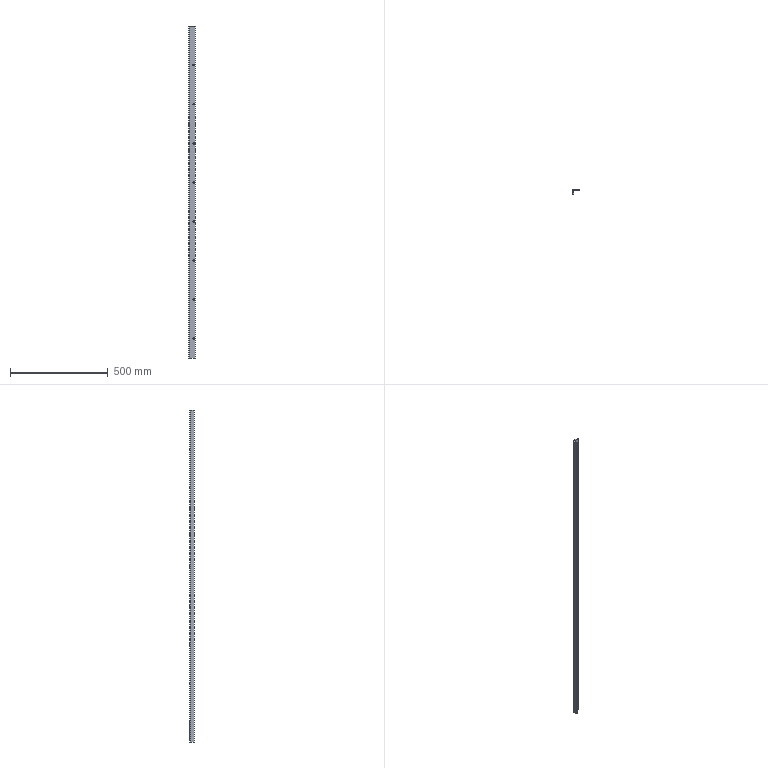Part | STEP file | Edge guard | 1 solid | 28 faces | box 35 x 25 x 1700 mm | volume 453852 mm3 | cylinder 19 | plane 9 | commonest cylinder face diameters 9 x17 1 x1 11 x1
STEP:
#1=CARTESIAN_POINT('',(7.,0.,-1895.5));
#2=VERTEX_POINT('',#1);
#3=CARTESIAN_POINT('',(7.,0.,-1904.5));
#4=VERTEX_POINT('',#3);
#5=CARTESIAN_POINT('',(7.,0.,-1900.));
#6=DIRECTION('',(0.,-1.,0.));
#7=DIRECTION('',(0.,0.,1.));
#8=AXIS2_PLACEMENT_3D('',#5,#6,#7);
#9=CIRCLE('',#8,4.5);
#10=EDGE_CURVE('',#2,#4,#9,.T.);
#11=ORIENTED_EDGE('',*,*,#10,.T.);
#12=CARTESIAN_POINT('',(7.,5.,-1904.5));
#13=VERTEX_POINT('',#12);
#14=CARTESIAN_POINT('',(7.,5.,-1904.5));
#15=DIRECTION('',(0.,1.,0.));
#16=VECTOR('',#15,1000.);
#17=LINE('',#14,#16);
#18=EDGE_CURVE('',#4,#13,#17,.T.);
#19=ORIENTED_EDGE('',*,*,#18,.T.);
#20=CARTESIAN_POINT('',(7.,5.,-1895.5));
#21=VERTEX_POINT('',#20);
#22=CARTESIAN_POINT('',(7.,5.,-1900.));
#23=DIRECTION('',(0.,-1.,0.));
#24=DIRECTION('',(0.,0.,1.));
#25=AXIS2_PLACEMENT_3D('',#22,#23,#24);
#26=CIRCLE('',#25,4.5);
#27=EDGE_CURVE('',#21,#13,#26,.T.);
#28=ORIENTED_EDGE('',*,*,#27,.F.);
#29=CARTESIAN_POINT('',(7.,5.,-1895.5));
#30=DIRECTION('',(0.,1.,0.));
#31=VECTOR('',#30,1000.);
#32=LINE('',#29,#31);
#33=EDGE_CURVE('',#2,#21,#32,.T.);
#34=ORIENTED_EDGE('',*,*,#33,.F.);
#35=EDGE_LOOP('',(#11,#19,#28,#34));
#36=FACE_OUTER_BOUND('',#35,.T.);
#37=CARTESIAN_POINT('',(7.,5.,-1900.));
#38=DIRECTION('',(0.,1.,0.));
#39=DIRECTION('',(0.,0.,1.));
#40=AXIS2_PLACEMENT_3D('',#37,#38,#39);
#41=CYLINDRICAL_SURFACE('',#40,4.5);
#42=ADVANCED_FACE('',(#36),#41,.F.);
#43=CARTESIAN_POINT('',(7.,0.,-1695.5));
#44=VERTEX_POINT('',#43);
#45=CARTESIAN_POINT('',(7.,0.,-1704.5));
#46=VERTEX_POINT('',#45);
#47=CARTESIAN_POINT('',(7.,0.,-1700.));
#48=DIRECTION('',(0.,-1.,0.));
#49=DIRECTION('',(0.,0.,1.));
#50=AXIS2_PLACEMENT_3D('',#47,#48,#49);
#51=CIRCLE('',#50,4.5);
#52=EDGE_CURVE('',#44,#46,#51,.T.);
#53=ORIENTED_EDGE('',*,*,#52,.T.);
#54=CARTESIAN_POINT('',(7.,5.,-1704.5));
#55=VERTEX_POINT('',#54);
#56=CARTESIAN_POINT('',(7.,5.,-1704.5));
#57=DIRECTION('',(0.,1.,0.));
#58=VECTOR('',#57,1000.);
#59=LINE('',#56,#58);
#60=EDGE_CURVE('',#46,#55,#59,.T.);
#61=ORIENTED_EDGE('',*,*,#60,.T.);
#62=CARTESIAN_POINT('',(7.,5.,-1695.5));
#63=VERTEX_POINT('',#62);
#64=CARTESIAN_POINT('',(7.,5.,-1700.));
#65=DIRECTION('',(0.,-1.,0.));
#66=DIRECTION('',(0.,0.,1.));
#67=AXIS2_PLACEMENT_3D('',#64,#65,#66);
#68=CIRCLE('',#67,4.5);
#69=EDGE_CURVE('',#63,#55,#68,.T.);
#70=ORIENTED_EDGE('',*,*,#69,.F.);
#71=CARTESIAN_POINT('',(7.,5.,-1695.5));
#72=DIRECTION('',(0.,1.,0.));
#73=VECTOR('',#72,1000.);
#74=LINE('',#71,#73);
#75=EDGE_CURVE('',#44,#63,#74,.T.);
#76=ORIENTED_EDGE('',*,*,#75,.F.);
#77=EDGE_LOOP('',(#53,#61,#70,#76));
#78=FACE_OUTER_BOUND('',#77,.T.);
#79=CARTESIAN_POINT('',(7.,5.,-1700.));
#80=DIRECTION('',(0.,1.,0.));
#81=DIRECTION('',(0.,0.,1.));
#82=AXIS2_PLACEMENT_3D('',#79,#80,#81);
#83=CYLINDRICAL_SURFACE('',#82,4.5);
#84=ADVANCED_FACE('',(#78),#83,.F.);
#85=CARTESIAN_POINT('',(7.,0.,-1495.5));
#86=VERTEX_POINT('',#85);
#87=CARTESIAN_POINT('',(7.,0.,-1504.5));
#88=VERTEX_POINT('',#87);
#89=CARTESIAN_POINT('',(7.,0.,-1500.));
#90=DIRECTION('',(0.,-1.,0.));
#91=DIRECTION('',(0.,0.,1.));
#92=AXIS2_PLACEMENT_3D('',#89,#90,#91);
#93=CIRCLE('',#92,4.5);
#94=EDGE_CURVE('',#86,#88,#93,.T.);
#95=ORIENTED_EDGE('',*,*,#94,.T.);
#96=CARTESIAN_POINT('',(7.,5.,-1504.5));
#97=VERTEX_POINT('',#96);
#98=CARTESIAN_POINT('',(7.,5.,-1504.5));
#99=DIRECTION('',(0.,1.,0.));
#100=VECTOR('',#99,1000.);
#101=LINE('',#98,#100);
#102=EDGE_CURVE('',#88,#97,#101,.T.);
#103=ORIENTED_EDGE('',*,*,#102,.T.);
#104=CARTESIAN_POINT('',(7.,5.,-1495.5));
#105=VERTEX_POINT('',#104);
#106=CARTESIAN_POINT('',(7.,5.,-1500.));
#107=DIRECTION('',(0.,-1.,0.));
#108=DIRECTION('',(0.,0.,1.));
#109=AXIS2_PLACEMENT_3D('',#106,#107,#108);
#110=CIRCLE('',#109,4.5);
#111=EDGE_CURVE('',#105,#97,#110,.T.);
#112=ORIENTED_EDGE('',*,*,#111,.F.);
#113=CARTESIAN_POINT('',(7.,5.,-1495.5));
#114=DIRECTION('',(0.,1.,0.));
#115=VECTOR('',#114,1000.);
#116=LINE('',#113,#115);
#117=EDGE_CURVE('',#86,#105,#116,.T.);
#118=ORIENTED_EDGE('',*,*,#117,.F.);
#119=EDGE_LOOP('',(#95,#103,#112,#118));
#120=FACE_OUTER_BOUND('',#119,.T.);
#121=CARTESIAN_POINT('',(7.,5.,-1500.));
#122=DIRECTION('',(0.,1.,0.));
#123=DIRECTION('',(0.,0.,1.));
#124=AXIS2_PLACEMENT_3D('',#121,#122,#123);
#125=CYLINDRICAL_SURFACE('',#124,4.5);
#126=ADVANCED_FACE('',(#120),#125,.F.);
#127=CARTESIAN_POINT('',(7.,0.,-1295.5));
#128=VERTEX_POINT('',#127);
#129=CARTESIAN_POINT('',(7.,0.,-1304.5));
#130=VERTEX_POINT('',#129);
#131=CARTESIAN_POINT('',(7.,0.,-1300.));
#132=DIRECTION('',(0.,-1.,0.));
#133=DIRECTION('',(0.,0.,1.));
#134=AXIS2_PLACEMENT_3D('',#131,#132,#133);
#135=CIRCLE('',#134,4.5);
#136=EDGE_CURVE('',#128,#130,#135,.T.);
#137=ORIENTED_EDGE('',*,*,#136,.T.);
#138=CARTESIAN_POINT('',(7.,5.,-1304.5));
#139=VERTEX_POINT('',#138);
#140=CARTESIAN_POINT('',(7.,5.,-1304.5));
#141=DIRECTION('',(0.,1.,0.));
#142=VECTOR('',#141,1000.);
#143=LINE('',#140,#142);
#144=EDGE_CURVE('',#130,#139,#143,.T.);
#145=ORIENTED_EDGE('',*,*,#144,.T.);
#146=CARTESIAN_POINT('',(7.,5.,-1295.5));
#147=VERTEX_POINT('',#146);
#148=CARTESIAN_POINT('',(7.,5.,-1300.));
#149=DIRECTION('',(0.,-1.,0.));
#150=DIRECTION('',(0.,0.,1.));
#151=AXIS2_PLACEMENT_3D('',#148,#149,#150);
#152=CIRCLE('',#151,4.5);
#153=EDGE_CURVE('',#147,#139,#152,.T.);
#154=ORIENTED_EDGE('',*,*,#153,.F.);
#155=CARTESIAN_POINT('',(7.,5.,-1295.5));
#156=DIRECTION('',(0.,1.,0.));
#157=VECTOR('',#156,1000.);
#158=LINE('',#155,#157);
#159=EDGE_CURVE('',#128,#147,#158,.T.);
#160=ORIENTED_EDGE('',*,*,#159,.F.);
#161=EDGE_LOOP('',(#137,#145,#154,#160));
#162=FACE_OUTER_BOUND('',#161,.T.);
#163=CARTESIAN_POINT('',(7.,5.,-1300.));
#164=DIRECTION('',(0.,1.,0.));
#165=DIRECTION('',(0.,0.,1.));
#166=AXIS2_PLACEMENT_3D('',#163,#164,#165);
#167=CYLINDRICAL_SURFACE('',#166,4.5);
#168=ADVANCED_FACE('',(#162),#167,.F.);
#169=CARTESIAN_POINT('',(7.,0.,-1095.5));
#170=VERTEX_POINT('',#169);
#171=CARTESIAN_POINT('',(7.,0.,-1104.5));
#172=VERTEX_POINT('',#171);
#173=CARTESIAN_POINT('',(7.,0.,-1100.));
#174=DIRECTION('',(0.,-1.,0.));
#175=DIRECTION('',(0.,0.,1.));
#176=AXIS2_PLACEMENT_3D('',#173,#174,#175);
#177=CIRCLE('',#176,4.5);
#178=EDGE_CURVE('',#170,#172,#177,.T.);
#179=ORIENTED_EDGE('',*,*,#178,.T.);
#180=CARTESIAN_POINT('',(7.,5.,-1104.5));
#181=VERTEX_POINT('',#180);
#182=CARTESIAN_POINT('',(7.,5.,-1104.5));
#183=DIRECTION('',(0.,1.,0.));
#184=VECTOR('',#183,1000.);
#185=LINE('',#182,#184);
#186=EDGE_CURVE('',#172,#181,#185,.T.);
#187=ORIENTED_EDGE('',*,*,#186,.T.);
#188=CARTESIAN_POINT('',(7.,5.,-1095.5));
#189=VERTEX_POINT('',#188);
#190=CARTESIAN_POINT('',(7.,5.,-1100.));
#191=DIRECTION('',(0.,-1.,0.));
#192=DIRECTION('',(0.,0.,1.));
#193=AXIS2_PLACEMENT_3D('',#190,#191,#192);
#194=CIRCLE('',#193,4.5);
#195=EDGE_CURVE('',#189,#181,#194,.T.);
#196=ORIENTED_EDGE('',*,*,#195,.F.);
#197=CARTESIAN_POINT('',(7.,5.,-1095.5));
#198=DIRECTION('',(0.,1.,0.));
#199=VECTOR('',#198,1000.);
#200=LINE('',#197,#199);
#201=EDGE_CURVE('',#170,#189,#200,.T.);
#202=ORIENTED_EDGE('',*,*,#201,.F.);
#203=EDGE_LOOP('',(#179,#187,#196,#202));
#204=FACE_OUTER_BOUND('',#203,.T.);
#205=CARTESIAN_POINT('',(7.,5.,-1100.));
#206=DIRECTION('',(0.,1.,0.));
#207=DIRECTION('',(0.,0.,1.));
#208=AXIS2_PLACEMENT_3D('',#205,#206,#207);
#209=CYLINDRICAL_SURFACE('',#208,4.5);
#210=ADVANCED_FACE('',(#204),#209,.F.);
#211=CARTESIAN_POINT('',(7.,0.,-895.5));
#212=VERTEX_POINT('',#211);
#213=CARTESIAN_POINT('',(7.,0.,-904.5));
#214=VERTEX_POINT('',#213);
#215=CARTESIAN_POINT('',(7.,0.,-900.));
#216=DIRECTION('',(0.,-1.,0.));
#217=DIRECTION('',(0.,0.,1.));
#218=AXIS2_PLACEMENT_3D('',#215,#216,#217);
#219=CIRCLE('',#218,4.5);
#220=EDGE_CURVE('',#212,#214,#219,.T.);
#221=ORIENTED_EDGE('',*,*,#220,.T.);
#222=CARTESIAN_POINT('',(7.,5.,-904.5));
#223=VERTEX_POINT('',#222);
#224=CARTESIAN_POINT('',(7.,5.,-904.5));
#225=DIRECTION('',(0.,1.,0.));
#226=VECTOR('',#225,1000.);
#227=LINE('',#224,#226);
#228=EDGE_CURVE('',#214,#223,#227,.T.);
#229=ORIENTED_EDGE('',*,*,#228,.T.);
#230=CARTESIAN_POINT('',(7.,5.,-895.5));
#231=VERTEX_POINT('',#230);
#232=CARTESIAN_POINT('',(7.,5.,-900.));
#233=DIRECTION('',(0.,-1.,0.));
#234=DIRECTION('',(0.,0.,1.));
#235=AXIS2_PLACEMENT_3D('',#232,#233,#234);
#236=CIRCLE('',#235,4.5);
#237=EDGE_CURVE('',#231,#223,#236,.T.);
#238=ORIENTED_EDGE('',*,*,#237,.F.);
#239=CARTESIAN_POINT('',(7.,5.,-895.5));
#240=DIRECTION('',(0.,1.,0.));
#241=VECTOR('',#240,1000.);
#242=LINE('',#239,#241);
#243=EDGE_CURVE('',#212,#231,#242,.T.);
#244=ORIENTED_EDGE('',*,*,#243,.F.);
#245=EDGE_LOOP('',(#221,#229,#238,#244));
#246=FACE_OUTER_BOUND('',#245,.T.);
#247=CARTESIAN_POINT('',(7.,5.,-900.));
#248=DIRECTION('',(0.,1.,0.));
#249=DIRECTION('',(0.,0.,1.));
#250=AXIS2_PLACEMENT_3D('',#247,#248,#249);
#251=CYLINDRICAL_SURFACE('',#250,4.5);
#252=ADVANCED_FACE('',(#246),#251,.F.);
#253=CARTESIAN_POINT('',(7.,0.,-695.5));
#254=VERTEX_POINT('',#253);
#255=CARTESIAN_POINT('',(7.,0.,-704.5));
#256=VERTEX_POINT('',#255);
#257=CARTESIAN_POINT('',(7.,0.,-700.));
#258=DIRECTION('',(0.,-1.,0.));
#259=DIRECTION('',(0.,0.,1.));
#260=AXIS2_PLACEMENT_3D('',#257,#258,#259);
#261=CIRCLE('',#260,4.5);
#262=EDGE_CURVE('',#254,#256,#261,.T.);
#263=ORIENTED_EDGE('',*,*,#262,.T.);
#264=CARTESIAN_POINT('',(7.,5.,-704.5));
#265=VERTEX_POINT('',#264);
#266=CARTESIAN_POINT('',(7.,5.,-704.5));
#267=DIRECTION('',(0.,1.,0.));
#268=VECTOR('',#267,1000.);
#269=LINE('',#266,#268);
#270=EDGE_CURVE('',#256,#265,#269,.T.);
#271=ORIENTED_EDGE('',*,*,#270,.T.);
#272=CARTESIAN_POINT('',(7.,5.,-695.5));
#273=VERTEX_POINT('',#272);
#274=CARTESIAN_POINT('',(7.,5.,-700.));
#275=DIRECTION('',(0.,-1.,0.));
#276=DIRECTION('',(0.,0.,1.));
#277=AXIS2_PLACEMENT_3D('',#274,#275,#276);
#278=CIRCLE('',#277,4.5);
#279=EDGE_CURVE('',#273,#265,#278,.T.);
#280=ORIENTED_EDGE('',*,*,#279,.F.);
#281=CARTESIAN_POINT('',(7.,5.,-695.5));
#282=DIRECTION('',(0.,1.,0.));
#283=VECTOR('',#282,1000.);
#284=LINE('',#281,#283);
#285=EDGE_CURVE('',#254,#273,#284,.T.);
#286=ORIENTED_EDGE('',*,*,#285,.F.);
#287=EDGE_LOOP('',(#263,#271,#280,#286));
#288=FACE_OUTER_BOUND('',#287,.T.);
#289=CARTESIAN_POINT('',(7.,5.,-700.));
#290=DIRECTION('',(0.,1.,0.));
#291=DIRECTION('',(0.,0.,1.));
#292=AXIS2_PLACEMENT_3D('',#289,#290,#291);
#293=CYLINDRICAL_SURFACE('',#292,4.5);
#294=ADVANCED_FACE('',(#288),#293,.F.);
#295=CARTESIAN_POINT('',(7.,0.,-495.5));
#296=VERTEX_POINT('',#295);
#297=CARTESIAN_POINT('',(7.,0.,-504.5));
#298=VERTEX_POINT('',#297);
#299=CARTESIAN_POINT('',(7.,0.,-500.));
#300=DIRECTION('',(0.,-1.,0.));
#301=DIRECTION('',(0.,0.,1.));
#302=AXIS2_PLACEMENT_3D('',#299,#300,#301);
#303=CIRCLE('',#302,4.5);
#304=EDGE_CURVE('',#296,#298,#303,.T.);
#305=ORIENTED_EDGE('',*,*,#304,.T.);
#306=CARTESIAN_POINT('',(7.,5.,-504.5));
#307=VERTEX_POINT('',#306);
#308=CARTESIAN_POINT('',(7.,5.,-504.5));
#309=DIRECTION('',(0.,1.,0.));
#310=VECTOR('',#309,1000.);
#311=LINE('',#308,#310);
#312=EDGE_CURVE('',#298,#307,#311,.T.);
#313=ORIENTED_EDGE('',*,*,#312,.T.);
#314=CARTESIAN_POINT('',(7.,5.,-495.5));
#315=VERTEX_POINT('',#314);
#316=CARTESIAN_POINT('',(7.,5.,-500.));
#317=DIRECTION('',(0.,-1.,0.));
#318=DIRECTION('',(0.,0.,1.));
#319=AXIS2_PLACEMENT_3D('',#316,#317,#318);
#320=CIRCLE('',#319,4.5);
#321=EDGE_CURVE('',#315,#307,#320,.T.);
#322=ORIENTED_EDGE('',*,*,#321,.F.);
#323=CARTESIAN_POINT('',(7.,5.,-495.5));
#324=DIRECTION('',(0.,1.,0.));
#325=VECTOR('',#324,1000.);
#326=LINE('',#323,#325);
#327=EDGE_CURVE('',#296,#315,#326,.T.);
#328=ORIENTED_EDGE('',*,*,#327,.F.);
#329=EDGE_LOOP('',(#305,#313,#322,#328));
#330=FACE_OUTER_BOUND('',#329,.T.);
#331=CARTESIAN_POINT('',(7.,5.,-500.));
#332=DIRECTION('',(0.,1.,0.));
#333=DIRECTION('',(0.,0.,1.));
#334=AXIS2_PLACEMENT_3D('',#331,#332,#333);
#335=CYLINDRICAL_SURFACE('',#334,4.5);
#336=ADVANCED_FACE('',(#330),#335,.F.);
#337=CARTESIAN_POINT('',(-20.,-20.,-2000.));
#338=VERTEX_POINT('',#337);
#339=CARTESIAN_POINT('',(-20.,-20.,-300.));
#340=VERTEX_POINT('',#339);
#341=CARTESIAN_POINT('',(-20.,-20.,-2000.));
#342=DIRECTION('',(0.,0.,1.));
#343=VECTOR('',#342,1000.);
#344=LINE('',#341,#343);
#345=EDGE_CURVE('',#338,#340,#344,.T.);
#346=ORIENTED_EDGE('',*,*,#345,.T.);
#347=CARTESIAN_POINT('',(-20.,-0.5,-300.));
#348=VERTEX_POINT('',#347);
#349=CARTESIAN_POINT('',(-20.,-0.5,-300.));
#350=DIRECTION('',(0.,-1.,0.));
#351=VECTOR('',#350,1000.);
#352=LINE('',#349,#351);
#353=EDGE_CURVE('',#348,#340,#352,.T.);
#354=ORIENTED_EDGE('',*,*,#353,.F.);
#355=CARTESIAN_POINT('',(-20.,-0.5,-2000.));
#356=VERTEX_POINT('',#355);
#357=CARTESIAN_POINT('',(-20.,-0.5,-2000.));
#358=DIRECTION('',(0.,0.,1.));
#359=VECTOR('',#358,1000.);
#360=LINE('',#357,#359);
#361=EDGE_CURVE('',#356,#348,#360,.T.);
#362=ORIENTED_EDGE('',*,*,#361,.F.);
#363=CARTESIAN_POINT('',(-20.,-0.5,-2000.));
#364=DIRECTION('',(0.,1.,0.));
#365=VECTOR('',#364,1000.);
#366=LINE('',#363,#365);
#367=EDGE_CURVE('',#338,#356,#366,.T.);
#368=ORIENTED_EDGE('',*,*,#367,.F.);
#369=EDGE_LOOP('',(#346,#354,#362,#368));
#370=FACE_OUTER_BOUND('',#369,.T.);
#371=CARTESIAN_POINT('',(-20.,0.,-2000.));
#372=DIRECTION('',(-1.,0.,0.));
#373=DIRECTION('',(0.,-1.,0.));
#374=AXIS2_PLACEMENT_3D('',#371,#372,#373);
#375=PLANE('',#374);
#376=ADVANCED_FACE('',(#370),#375,.T.);
#377=CARTESIAN_POINT('',(-15.,-20.,-300.));
#378=VERTEX_POINT('',#377);
#379=CARTESIAN_POINT('',(-20.,-20.,-300.));
#380=DIRECTION('',(1.,0.,0.));
#381=VECTOR('',#380,1000.);
#382=LINE('',#379,#381);
#383=EDGE_CURVE('',#340,#378,#382,.T.);
#384=ORIENTED_EDGE('',*,*,#383,.F.);
#385=ORIENTED_EDGE('',*,*,#345,.F.);
#386=CARTESIAN_POINT('',(-15.,-20.,-2000.));
#387=VERTEX_POINT('',#386);
#388=CARTESIAN_POINT('',(-15.,-20.,-2000.));
#389=DIRECTION('',(-1.,0.,0.));
#390=VECTOR('',#389,1000.);
#391=LINE('',#388,#390);
#392=EDGE_CURVE('',#387,#338,#391,.T.);
#393=ORIENTED_EDGE('',*,*,#392,.F.);
#394=CARTESIAN_POINT('',(-15.,-20.,-2000.));
#395=DIRECTION('',(0.,0.,1.));
#396=VECTOR('',#395,1000.);
#397=LINE('',#394,#396);
#398=EDGE_CURVE('',#387,#378,#397,.T.);
#399=ORIENTED_EDGE('',*,*,#398,.T.);
#400=EDGE_LOOP('',(#384,#385,#393,#399));
#401=FACE_OUTER_BOUND('',#400,.T.);
#402=CARTESIAN_POINT('',(-15.,-20.,-2000.));
#403=DIRECTION('',(0.,1.,0.));
#404=DIRECTION('',(0.,0.,1.));
#405=AXIS2_PLACEMENT_3D('',#402,#403,#404);
#406=PLANE('',#405);
#407=ADVANCED_FACE('',(#401),#406,.F.);
#408=ORIENTED_EDGE('',*,*,#361,.T.);
#409=CARTESIAN_POINT('',(-14.5,5.,-300.));
#410=VERTEX_POINT('',#409);
#411=CARTESIAN_POINT('',(-14.5,-0.5,-300.));
#412=DIRECTION('',(0.,0.,1.));
#413=DIRECTION('',(1.,0.,0.));
#414=AXIS2_PLACEMENT_3D('',#411,#412,#413);
#415=CIRCLE('',#414,5.5);
#416=EDGE_CURVE('',#410,#348,#415,.T.);
#417=ORIENTED_EDGE('',*,*,#416,.F.);
#418=CARTESIAN_POINT('',(-14.5,5.,-2000.));
#419=VERTEX_POINT('',#418);
#420=CARTESIAN_POINT('',(-14.5,5.,-2000.));
#421=DIRECTION('',(0.,0.,1.));
#422=VECTOR('',#421,1000.);
#423=LINE('',#420,#422);
#424=EDGE_CURVE('',#419,#410,#423,.T.);
#425=ORIENTED_EDGE('',*,*,#424,.F.);
#426=CARTESIAN_POINT('',(-14.5,-0.5,-2000.));
#427=DIRECTION('',(0.,0.,-1.));
#428=DIRECTION('',(1.,0.,0.));
#429=AXIS2_PLACEMENT_3D('',#426,#427,#428);
#430=CIRCLE('',#429,5.5);
#431=EDGE_CURVE('',#356,#419,#430,.T.);
#432=ORIENTED_EDGE('',*,*,#431,.F.);
#433=EDGE_LOOP('',(#408,#417,#425,#432));
#434=FACE_OUTER_BOUND('',#433,.T.);
#435=CARTESIAN_POINT('',(-14.5,-0.5,-2000.));
#436=DIRECTION('',(0.,0.,1.));
#437=DIRECTION('',(1.,0.,0.));
#438=AXIS2_PLACEMENT_3D('',#435,#436,#437);
#439=CYLINDRICAL_SURFACE('',#438,5.5);
#440=ADVANCED_FACE('',(#434),#439,.T.);
#441=CARTESIAN_POINT('',(-15.,-0.5,-300.));
#442=VERTEX_POINT('',#441);
#443=CARTESIAN_POINT('',(-15.,-20.,-300.));
#444=DIRECTION('',(0.,1.,0.));
#445=VECTOR('',#444,1000.);
#446=LINE('',#443,#445);
#447=EDGE_CURVE('',#378,#442,#446,.T.);
#448=ORIENTED_EDGE('',*,*,#447,.F.);
#449=ORIENTED_EDGE('',*,*,#398,.F.);
#450=CARTESIAN_POINT('',(-15.,-0.5,-2000.));
#451=VERTEX_POINT('',#450);
#452=CARTESIAN_POINT('',(-15.,0.,-2000.));
#453=DIRECTION('',(0.,-1.,0.));
#454=VECTOR('',#453,1000.);
#455=LINE('',#452,#454);
#456=EDGE_CURVE('',#451,#387,#455,.T.);
#457=ORIENTED_EDGE('',*,*,#456,.F.);
#458=CARTESIAN_POINT('',(-15.,-0.5,-2000.));
#459=DIRECTION('',(0.,0.,1.));
#460=VECTOR('',#459,1000.);
#461=LINE('',#458,#460);
#462=EDGE_CURVE('',#451,#442,#461,.T.);
#463=ORIENTED_EDGE('',*,*,#462,.T.);
#464=EDGE_LOOP('',(#448,#449,#457,#463));
#465=FACE_OUTER_BOUND('',#464,.T.);
#466=CARTESIAN_POINT('',(-15.,0.,-2000.));
#467=DIRECTION('',(-1.,0.,0.));
#468=DIRECTION('',(0.,-1.,0.));
#469=AXIS2_PLACEMENT_3D('',#466,#467,#468);
#470=PLANE('',#469);
#471=ADVANCED_FACE('',(#465),#470,.F.);
#472=ORIENTED_EDGE('',*,*,#321,.T.);
#473=CARTESIAN_POINT('',(7.,5.,-500.));
#474=DIRECTION('',(0.,-1.,0.));
#475=DIRECTION('',(0.,0.,1.));
#476=AXIS2_PLACEMENT_3D('',#473,#474,#475);
#477=CIRCLE('',#476,4.5);
#478=EDGE_CURVE('',#307,#315,#477,.T.);
#479=ORIENTED_EDGE('',*,*,#478,.T.);
#480=EDGE_LOOP('',(#472,#479));
#481=FACE_BOUND('',#480,.T.);
#482=ORIENTED_EDGE('',*,*,#279,.T.);
#483=CARTESIAN_POINT('',(7.,5.,-700.));
#484=DIRECTION('',(0.,-1.,0.));
#485=DIRECTION('',(0.,0.,1.));
#486=AXIS2_PLACEMENT_3D('',#483,#484,#485);
#487=CIRCLE('',#486,4.5);
#488=EDGE_CURVE('',#265,#273,#487,.T.);
#489=ORIENTED_EDGE('',*,*,#488,.T.);
#490=EDGE_LOOP('',(#482,#489));
#491=FACE_BOUND('',#490,.T.);
#492=ORIENTED_EDGE('',*,*,#237,.T.);
#493=CARTESIAN_POINT('',(7.,5.,-900.));
#494=DIRECTION('',(0.,-1.,0.));
#495=DIRECTION('',(0.,0.,1.));
#496=AXIS2_PLACEMENT_3D('',#493,#494,#495);
#497=CIRCLE('',#496,4.5);
#498=EDGE_CURVE('',#223,#231,#497,.T.);
#499=ORIENTED_EDGE('',*,*,#498,.T.);
#500=EDGE_LOOP('',(#492,#499));
#501=FACE_BOUND('',#500,.T.);
#502=ORIENTED_EDGE('',*,*,#195,.T.);
#503=CARTESIAN_POINT('',(7.,5.,-1100.));
#504=DIRECTION('',(0.,-1.,0.));
#505=DIRECTION('',(0.,0.,1.));
#506=AXIS2_PLACEMENT_3D('',#503,#504,#505);
#507=CIRCLE('',#506,4.5);
#508=EDGE_CURVE('',#181,#189,#507,.T.);
#509=ORIENTED_EDGE('',*,*,#508,.T.);
#510=EDGE_LOOP('',(#502,#509));
#511=FACE_BOUND('',#510,.T.);
#512=ORIENTED_EDGE('',*,*,#153,.T.);
#513=CARTESIAN_POINT('',(7.,5.,-1300.));
#514=DIRECTION('',(0.,-1.,0.));
#515=DIRECTION('',(0.,0.,1.));
#516=AXIS2_PLACEMENT_3D('',#513,#514,#515);
#517=CIRCLE('',#516,4.5);
#518=EDGE_CURVE('',#139,#147,#517,.T.);
#519=ORIENTED_EDGE('',*,*,#518,.T.);
#520=EDGE_LOOP('',(#512,#519));
#521=FACE_BOUND('',#520,.T.);
#522=ORIENTED_EDGE('',*,*,#111,.T.);
#523=CARTESIAN_POINT('',(7.,5.,-1500.));
#524=DIRECTION('',(0.,-1.,0.));
#525=DIRECTION('',(0.,0.,1.));
#526=AXIS2_PLACEMENT_3D('',#523,#524,#525);
#527=CIRCLE('',#526,4.5);
#528=EDGE_CURVE('',#97,#105,#527,.T.);
#529=ORIENTED_EDGE('',*,*,#528,.T.);
#530=EDGE_LOOP('',(#522,#529));
#531=FACE_BOUND('',#530,.T.);
#532=ORIENTED_EDGE('',*,*,#69,.T.);
#533=CARTESIAN_POINT('',(7.,5.,-1700.));
#534=DIRECTION('',(0.,-1.,0.));
#535=DIRECTION('',(0.,0.,1.));
#536=AXIS2_PLACEMENT_3D('',#533,#534,#535);
#537=CIRCLE('',#536,4.5);
#538=EDGE_CURVE('',#55,#63,#537,.T.);
#539=ORIENTED_EDGE('',*,*,#538,.T.);
#540=EDGE_LOOP('',(#532,#539));
#541=FACE_BOUND('',#540,.T.);
#542=ORIENTED_EDGE('',*,*,#27,.T.);
#543=CARTESIAN_POINT('',(7.,5.,-1900.));
#544=DIRECTION('',(0.,-1.,0.));
#545=DIRECTION('',(0.,0.,1.));
#546=AXIS2_PLACEMENT_3D('',#543,#544,#545);
#547=CIRCLE('',#546,4.5);
#548=EDGE_CURVE('',#13,#21,#547,.T.);
#549=ORIENTED_EDGE('',*,*,#548,.T.);
#550=EDGE_LOOP('',(#542,#549));
#551=FACE_BOUND('',#550,.T.);
#552=ORIENTED_EDGE('',*,*,#424,.T.);
#553=CARTESIAN_POINT('',(2.5,5.,-300.));
#554=VERTEX_POINT('',#553);
#555=CARTESIAN_POINT('',(15.,5.,-300.));
#556=DIRECTION('',(-1.,0.,0.));
#557=VECTOR('',#556,1000.);
#558=LINE('',#555,#557);
#559=EDGE_CURVE('',#554,#410,#558,.T.);
#560=ORIENTED_EDGE('',*,*,#559,.F.);
#561=CARTESIAN_POINT('',(11.5,5.,-300.));
#562=VERTEX_POINT('',#561);
#563=CARTESIAN_POINT('',(7.,5.,-300.));
#564=DIRECTION('',(0.,-1.,0.));
#565=DIRECTION('',(0.,0.,1.));
#566=AXIS2_PLACEMENT_3D('',#563,#564,#565);
#567=CIRCLE('',#566,4.5);
#568=EDGE_CURVE('',#554,#562,#567,.T.);
#569=ORIENTED_EDGE('',*,*,#568,.T.);
#570=CARTESIAN_POINT('',(15.,5.,-300.));
#571=VERTEX_POINT('',#570);
#572=CARTESIAN_POINT('',(15.,5.,-300.));
#573=DIRECTION('',(-1.,0.,0.));
#574=VECTOR('',#573,1000.);
#575=LINE('',#572,#574);
#576=EDGE_CURVE('',#571,#562,#575,.T.);
#577=ORIENTED_EDGE('',*,*,#576,.F.);
#578=CARTESIAN_POINT('',(15.,5.,-2000.));
#579=VERTEX_POINT('',#578);
#580=CARTESIAN_POINT('',(15.,5.,-2000.));
#581=DIRECTION('',(0.,0.,-1.));
#582=VECTOR('',#581,1000.);
#583=LINE('',#580,#582);
#584=EDGE_CURVE('',#571,#579,#583,.T.);
#585=ORIENTED_EDGE('',*,*,#584,.T.);
#586=CARTESIAN_POINT('',(-20.,5.,-2000.));
#587=DIRECTION('',(1.,0.,0.));
#588=VECTOR('',#587,1000.);
#589=LINE('',#586,#588);
#590=EDGE_CURVE('',#419,#579,#589,.T.);
#591=ORIENTED_EDGE('',*,*,#590,.F.);
#592=EDGE_LOOP('',(#552,#560,#569,#577,#585,#591));
#593=FACE_OUTER_BOUND('',#592,.T.);
#594=CARTESIAN_POINT('',(15.,5.,-2000.));
#595=DIRECTION('',(0.,1.,0.));
#596=DIRECTION('',(0.,0.,1.));
#597=AXIS2_PLACEMENT_3D('',#594,#595,#596);
#598=PLANE('',#597);
#599=ADVANCED_FACE('',(#481,#491,#501,#511,#521,#531,#541,#551,#593),#598,.T.);
#600=CARTESIAN_POINT('',(11.5,0.,-300.));
#601=VERTEX_POINT('',#600);
#602=CARTESIAN_POINT('',(11.5,5.,-300.));
#603=DIRECTION('',(0.,-1.,0.));
#604=VECTOR('',#603,1000.);
#605=LINE('',#602,#604);
#606=EDGE_CURVE('',#562,#601,#605,.T.);
#607=ORIENTED_EDGE('',*,*,#606,.F.);
#608=ORIENTED_EDGE('',*,*,#568,.F.);
#609=CARTESIAN_POINT('',(2.5,0.,-300.));
#610=VERTEX_POINT('',#609);
#611=CARTESIAN_POINT('',(2.5,5.,-300.));
#612=DIRECTION('',(0.,1.,0.));
#613=VECTOR('',#612,1000.);
#614=LINE('',#611,#613);
#615=EDGE_CURVE('',#610,#554,#614,.T.);
#616=ORIENTED_EDGE('',*,*,#615,.F.);
#617=CARTESIAN_POINT('',(7.,0.,-300.));
#618=DIRECTION('',(0.,-1.,0.));
#619=DIRECTION('',(0.,0.,1.));
#620=AXIS2_PLACEMENT_3D('',#617,#618,#619);
#621=CIRCLE('',#620,4.5);
#622=EDGE_CURVE('',#610,#601,#621,.T.);
#623=ORIENTED_EDGE('',*,*,#622,.T.);
#624=EDGE_LOOP('',(#607,#608,#616,#623));
#625=FACE_OUTER_BOUND('',#624,.T.);
#626=CARTESIAN_POINT('',(7.,5.,-300.));
#627=DIRECTION('',(0.,1.,0.));
#628=DIRECTION('',(0.,0.,1.));
#629=AXIS2_PLACEMENT_3D('',#626,#627,#628);
#630=CYLINDRICAL_SURFACE('',#629,4.5);
#631=ADVANCED_FACE('',(#625),#630,.F.);
#632=CARTESIAN_POINT('',(15.,0.,-300.));
#633=VERTEX_POINT('',#632);
#634=CARTESIAN_POINT('',(15.,0.,-300.));
#635=DIRECTION('',(0.,1.,0.));
#636=VECTOR('',#635,1000.);
#637=LINE('',#634,#636);
#638=EDGE_CURVE('',#633,#571,#637,.T.);
#639=ORIENTED_EDGE('',*,*,#638,.F.);
#640=CARTESIAN_POINT('',(15.,0.,-2000.));
#641=VERTEX_POINT('',#640);
#642=CARTESIAN_POINT('',(15.,0.,-2000.));
#643=DIRECTION('',(0.,0.,-1.));
#644=VECTOR('',#643,1000.);
#645=LINE('',#642,#644);
#646=EDGE_CURVE('',#633,#641,#645,.T.);
#647=ORIENTED_EDGE('',*,*,#646,.T.);
#648=CARTESIAN_POINT('',(15.,-0.5,-2000.));
#649=DIRECTION('',(0.,-1.,0.));
#650=VECTOR('',#649,1000.);
#651=LINE('',#648,#650);
#652=EDGE_CURVE('',#579,#641,#651,.T.);
#653=ORIENTED_EDGE('',*,*,#652,.F.);
#654=ORIENTED_EDGE('',*,*,#584,.F.);
#655=EDGE_LOOP('',(#639,#647,#653,#654));
#656=FACE_OUTER_BOUND('',#655,.T.);
#657=CARTESIAN_POINT('',(15.,5.,-2000.));
#658=DIRECTION('',(-1.,0.,0.));
#659=DIRECTION('',(0.,0.,1.));
#660=AXIS2_PLACEMENT_3D('',#657,#658,#659);
#661=PLANE('',#660);
#662=ADVANCED_FACE('',(#656),#661,.F.);
#663=CARTESIAN_POINT('',(-14.5,0.,-300.));
#664=VERTEX_POINT('',#663);
#665=CARTESIAN_POINT('',(-14.5,-0.5,-300.));
#666=DIRECTION('',(0.,0.,-1.));
#667=DIRECTION('',(1.,0.,0.));
#668=AXIS2_PLACEMENT_3D('',#665,#666,#667);
#669=CIRCLE('',#668,0.5);
#670=EDGE_CURVE('',#442,#664,#669,.T.);
#671=ORIENTED_EDGE('',*,*,#670,.F.);
#672=ORIENTED_EDGE('',*,*,#462,.F.);
#673=CARTESIAN_POINT('',(-14.5,0.,-2000.));
#674=VERTEX_POINT('',#673);
#675=CARTESIAN_POINT('',(-14.5,-0.5,-2000.));
#676=DIRECTION('',(0.,0.,1.));
#677=DIRECTION('',(1.,0.,0.));
#678=AXIS2_PLACEMENT_3D('',#675,#676,#677);
#679=CIRCLE('',#678,0.5);
#680=EDGE_CURVE('',#674,#451,#679,.T.);
#681=ORIENTED_EDGE('',*,*,#680,.F.);
#682=CARTESIAN_POINT('',(-14.5,0.,-2000.));
#683=DIRECTION('',(0.,0.,1.));
#684=VECTOR('',#683,1000.);
#685=LINE('',#682,#684);
#686=EDGE_CURVE('',#674,#664,#685,.T.);
#687=ORIENTED_EDGE('',*,*,#686,.T.);
#688=EDGE_LOOP('',(#671,#672,#681,#687));
#689=FACE_OUTER_BOUND('',#688,.T.);
#690=CARTESIAN_POINT('',(-14.5,-0.5,-2000.));
#691=DIRECTION('',(0.,0.,1.));
#692=DIRECTION('',(1.,0.,0.));
#693=AXIS2_PLACEMENT_3D('',#690,#691,#692);
#694=CYLINDRICAL_SURFACE('',#693,0.5);
#695=ADVANCED_FACE('',(#689),#694,.F.);
#696=ORIENTED_EDGE('',*,*,#304,.F.);
#697=CARTESIAN_POINT('',(7.,0.,-500.));
#698=DIRECTION('',(0.,-1.,0.));
#699=DIRECTION('',(0.,0.,1.));
#700=AXIS2_PLACEMENT_3D('',#697,#698,#699);
#701=CIRCLE('',#700,4.5);
#702=EDGE_CURVE('',#298,#296,#701,.T.);
#703=ORIENTED_EDGE('',*,*,#702,.F.);
#704=EDGE_LOOP('',(#696,#703));
#705=FACE_BOUND('',#704,.T.);
#706=ORIENTED_EDGE('',*,*,#262,.F.);
#707=CARTESIAN_POINT('',(7.,0.,-700.));
#708=DIRECTION('',(0.,-1.,0.));
#709=DIRECTION('',(0.,0.,1.));
#710=AXIS2_PLACEMENT_3D('',#707,#708,#709);
#711=CIRCLE('',#710,4.5);
#712=EDGE_CURVE('',#256,#254,#711,.T.);
#713=ORIENTED_EDGE('',*,*,#712,.F.);
#714=EDGE_LOOP('',(#706,#713));
#715=FACE_BOUND('',#714,.T.);
#716=ORIENTED_EDGE('',*,*,#220,.F.);
#717=CARTESIAN_POINT('',(7.,0.,-900.));
#718=DIRECTION('',(0.,-1.,0.));
#719=DIRECTION('',(0.,0.,1.));
#720=AXIS2_PLACEMENT_3D('',#717,#718,#719);
#721=CIRCLE('',#720,4.5);
#722=EDGE_CURVE('',#214,#212,#721,.T.);
#723=ORIENTED_EDGE('',*,*,#722,.F.);
#724=EDGE_LOOP('',(#716,#723));
#725=FACE_BOUND('',#724,.T.);
#726=ORIENTED_EDGE('',*,*,#178,.F.);
#727=CARTESIAN_POINT('',(7.,0.,-1100.));
#728=DIRECTION('',(0.,-1.,0.));
#729=DIRECTION('',(0.,0.,1.));
#730=AXIS2_PLACEMENT_3D('',#727,#728,#729);
#731=CIRCLE('',#730,4.5);
#732=EDGE_CURVE('',#172,#170,#731,.T.);
#733=ORIENTED_EDGE('',*,*,#732,.F.);
#734=EDGE_LOOP('',(#726,#733));
#735=FACE_BOUND('',#734,.T.);
#736=ORIENTED_EDGE('',*,*,#136,.F.);
#737=CARTESIAN_POINT('',(7.,0.,-1300.));
#738=DIRECTION('',(0.,-1.,0.));
#739=DIRECTION('',(0.,0.,1.));
#740=AXIS2_PLACEMENT_3D('',#737,#738,#739);
#741=CIRCLE('',#740,4.5);
#742=EDGE_CURVE('',#130,#128,#741,.T.);
#743=ORIENTED_EDGE('',*,*,#742,.F.);
#744=EDGE_LOOP('',(#736,#743));
#745=FACE_BOUND('',#744,.T.);
#746=ORIENTED_EDGE('',*,*,#94,.F.);
#747=CARTESIAN_POINT('',(7.,0.,-1500.));
#748=DIRECTION('',(0.,-1.,0.));
#749=DIRECTION('',(0.,0.,1.));
#750=AXIS2_PLACEMENT_3D('',#747,#748,#749);
#751=CIRCLE('',#750,4.5);
#752=EDGE_CURVE('',#88,#86,#751,.T.);
#753=ORIENTED_EDGE('',*,*,#752,.F.);
#754=EDGE_LOOP('',(#746,#753));
#755=FACE_BOUND('',#754,.T.);
#756=ORIENTED_EDGE('',*,*,#52,.F.);
#757=CARTESIAN_POINT('',(7.,0.,-1700.));
#758=DIRECTION('',(0.,-1.,0.));
#759=DIRECTION('',(0.,0.,1.));
#760=AXIS2_PLACEMENT_3D('',#757,#758,#759);
#761=CIRCLE('',#760,4.5);
#762=EDGE_CURVE('',#46,#44,#761,.T.);
#763=ORIENTED_EDGE('',*,*,#762,.F.);
#764=EDGE_LOOP('',(#756,#763));
#765=FACE_BOUND('',#764,.T.);
#766=ORIENTED_EDGE('',*,*,#10,.F.);
#767=CARTESIAN_POINT('',(7.,0.,-1900.));
#768=DIRECTION('',(0.,-1.,0.));
#769=DIRECTION('',(0.,0.,1.));
#770=AXIS2_PLACEMENT_3D('',#767,#768,#769);
#771=CIRCLE('',#770,4.5);
#772=EDGE_CURVE('',#4,#2,#771,.T.);
#773=ORIENTED_EDGE('',*,*,#772,.F.);
#774=EDGE_LOOP('',(#766,#773));
#775=FACE_BOUND('',#774,.T.);
#776=CARTESIAN_POINT('',(-14.5,0.,-300.));
#777=DIRECTION('',(1.,0.,0.));
#778=VECTOR('',#777,1000.);
#779=LINE('',#776,#778);
#780=EDGE_CURVE('',#664,#610,#779,.T.);
#781=ORIENTED_EDGE('',*,*,#780,.F.);
#782=ORIENTED_EDGE('',*,*,#686,.F.);
#783=CARTESIAN_POINT('',(15.,0.,-2000.));
#784=DIRECTION('',(-1.,0.,0.));
#785=VECTOR('',#784,1000.);
#786=LINE('',#783,#785);
#787=EDGE_CURVE('',#641,#674,#786,.T.);
#788=ORIENTED_EDGE('',*,*,#787,.F.);
#789=ORIENTED_EDGE('',*,*,#646,.F.);
#790=CARTESIAN_POINT('',(15.,0.,-300.));
#791=DIRECTION('',(1.,0.,0.));
#792=VECTOR('',#791,1000.);
#793=LINE('',#790,#792);
#794=EDGE_CURVE('',#601,#633,#793,.T.);
#795=ORIENTED_EDGE('',*,*,#794,.F.);
#796=ORIENTED_EDGE('',*,*,#622,.F.);
#797=EDGE_LOOP('',(#781,#782,#788,#789,#795,#796));
#798=FACE_OUTER_BOUND('',#797,.T.);
#799=CARTESIAN_POINT('',(15.,0.,-2000.));
#800=DIRECTION('',(0.,1.,0.));
#801=DIRECTION('',(0.,0.,1.));
#802=AXIS2_PLACEMENT_3D('',#799,#800,#801);
#803=PLANE('',#802);
#804=ADVANCED_FACE('',(#705,#715,#725,#735,#745,#755,#765,#775,#798),#803,.F.);
#805=ORIENTED_EDGE('',*,*,#590,.T.);
#806=ORIENTED_EDGE('',*,*,#652,.T.);
#807=ORIENTED_EDGE('',*,*,#787,.T.);
#808=ORIENTED_EDGE('',*,*,#680,.T.);
#809=ORIENTED_EDGE('',*,*,#456,.T.);
#810=ORIENTED_EDGE('',*,*,#392,.T.);
#811=ORIENTED_EDGE('',*,*,#367,.T.);
#812=ORIENTED_EDGE('',*,*,#431,.T.);
#813=EDGE_LOOP('',(#805,#806,#807,#808,#809,#810,#811,#812));
#814=FACE_OUTER_BOUND('',#813,.T.);
#815=CARTESIAN_POINT('',(-20.,-0.5,-2000.));
#816=DIRECTION('',(0.,0.,-1.));
#817=DIRECTION('',(-1.,0.,0.));
#818=AXIS2_PLACEMENT_3D('',#815,#816,#817);
#819=PLANE('',#818);
#820=ADVANCED_FACE('',(#814),#819,.T.);
#821=ORIENTED_EDGE('',*,*,#18,.F.);
#822=ORIENTED_EDGE('',*,*,#772,.T.);
#823=ORIENTED_EDGE('',*,*,#33,.T.);
#824=ORIENTED_EDGE('',*,*,#548,.F.);
#825=EDGE_LOOP('',(#821,#822,#823,#824));
#826=FACE_OUTER_BOUND('',#825,.T.);
#827=CARTESIAN_POINT('',(7.,5.,-1900.));
#828=DIRECTION('',(0.,1.,0.));
#829=DIRECTION('',(0.,0.,1.));
#830=AXIS2_PLACEMENT_3D('',#827,#828,#829);
#831=CYLINDRICAL_SURFACE('',#830,4.5);
#832=ADVANCED_FACE('',(#826),#831,.F.);
#833=ORIENTED_EDGE('',*,*,#60,.F.);
#834=ORIENTED_EDGE('',*,*,#762,.T.);
#835=ORIENTED_EDGE('',*,*,#75,.T.);
#836=ORIENTED_EDGE('',*,*,#538,.F.);
#837=EDGE_LOOP('',(#833,#834,#835,#836));
#838=FACE_OUTER_BOUND('',#837,.T.);
#839=CARTESIAN_POINT('',(7.,5.,-1700.));
#840=DIRECTION('',(0.,1.,0.));
#841=DIRECTION('',(0.,0.,1.));
#842=AXIS2_PLACEMENT_3D('',#839,#840,#841);
#843=CYLINDRICAL_SURFACE('',#842,4.5);
#844=ADVANCED_FACE('',(#838),#843,.F.);
#845=ORIENTED_EDGE('',*,*,#102,.F.);
#846=ORIENTED_EDGE('',*,*,#752,.T.);
#847=ORIENTED_EDGE('',*,*,#117,.T.);
#848=ORIENTED_EDGE('',*,*,#528,.F.);
#849=EDGE_LOOP('',(#845,#846,#847,#848));
#850=FACE_OUTER_BOUND('',#849,.T.);
#851=CARTESIAN_POINT('',(7.,5.,-1500.));
#852=DIRECTION('',(0.,1.,0.));
#853=DIRECTION('',(0.,0.,1.));
#854=AXIS2_PLACEMENT_3D('',#851,#852,#853);
#855=CYLINDRICAL_SURFACE('',#854,4.5);
#856=ADVANCED_FACE('',(#850),#855,.F.);
#857=ORIENTED_EDGE('',*,*,#144,.F.);
#858=ORIENTED_EDGE('',*,*,#742,.T.);
#859=ORIENTED_EDGE('',*,*,#159,.T.);
#860=ORIENTED_EDGE('',*,*,#518,.F.);
#861=EDGE_LOOP('',(#857,#858,#859,#860));
#862=FACE_OUTER_BOUND('',#861,.T.);
#863=CARTESIAN_POINT('',(7.,5.,-1300.));
#864=DIRECTION('',(0.,1.,0.));
#865=DIRECTION('',(0.,0.,1.));
#866=AXIS2_PLACEMENT_3D('',#863,#864,#865);
#867=CYLINDRICAL_SURFACE('',#866,4.5);
#868=ADVANCED_FACE('',(#862),#867,.F.);
#869=ORIENTED_EDGE('',*,*,#186,.F.);
#870=ORIENTED_EDGE('',*,*,#732,.T.);
#871=ORIENTED_EDGE('',*,*,#201,.T.);
#872=ORIENTED_EDGE('',*,*,#508,.F.);
#873=EDGE_LOOP('',(#869,#870,#871,#872));
#874=FACE_OUTER_BOUND('',#873,.T.);
#875=CARTESIAN_POINT('',(7.,5.,-1100.));
#876=DIRECTION('',(0.,1.,0.));
#877=DIRECTION('',(0.,0.,1.));
#878=AXIS2_PLACEMENT_3D('',#875,#876,#877);
#879=CYLINDRICAL_SURFACE('',#878,4.5);
#880=ADVANCED_FACE('',(#874),#879,.F.);
#881=ORIENTED_EDGE('',*,*,#228,.F.);
#882=ORIENTED_EDGE('',*,*,#722,.T.);
#883=ORIENTED_EDGE('',*,*,#243,.T.);
#884=ORIENTED_EDGE('',*,*,#498,.F.);
#885=EDGE_LOOP('',(#881,#882,#883,#884));
#886=FACE_OUTER_BOUND('',#885,.T.);
#887=CARTESIAN_POINT('',(7.,5.,-900.));
#888=DIRECTION('',(0.,1.,0.));
#889=DIRECTION('',(0.,0.,1.));
#890=AXIS2_PLACEMENT_3D('',#887,#888,#889);
#891=CYLINDRICAL_SURFACE('',#890,4.5);
#892=ADVANCED_FACE('',(#886),#891,.F.);
#893=ORIENTED_EDGE('',*,*,#270,.F.);
#894=ORIENTED_EDGE('',*,*,#712,.T.);
#895=ORIENTED_EDGE('',*,*,#285,.T.);
#896=ORIENTED_EDGE('',*,*,#488,.F.);
#897=EDGE_LOOP('',(#893,#894,#895,#896));
#898=FACE_OUTER_BOUND('',#897,.T.);
#899=CARTESIAN_POINT('',(7.,5.,-700.));
#900=DIRECTION('',(0.,1.,0.));
#901=DIRECTION('',(0.,0.,1.));
#902=AXIS2_PLACEMENT_3D('',#899,#900,#901);
#903=CYLINDRICAL_SURFACE('',#902,4.5);
#904=ADVANCED_FACE('',(#898),#903,.F.);
#905=ORIENTED_EDGE('',*,*,#312,.F.);
#906=ORIENTED_EDGE('',*,*,#702,.T.);
#907=ORIENTED_EDGE('',*,*,#327,.T.);
#908=ORIENTED_EDGE('',*,*,#478,.F.);
#909=EDGE_LOOP('',(#905,#906,#907,#908));
#910=FACE_OUTER_BOUND('',#909,.T.);
#911=CARTESIAN_POINT('',(7.,5.,-500.));
#912=DIRECTION('',(0.,1.,0.));
#913=DIRECTION('',(0.,0.,1.));
#914=AXIS2_PLACEMENT_3D('',#911,#912,#913);
#915=CYLINDRICAL_SURFACE('',#914,4.5);
#916=ADVANCED_FACE('',(#910),#915,.F.);
#917=ORIENTED_EDGE('',*,*,#606,.T.);
#918=ORIENTED_EDGE('',*,*,#794,.T.);
#919=ORIENTED_EDGE('',*,*,#638,.T.);
#920=ORIENTED_EDGE('',*,*,#576,.T.);
#921=EDGE_LOOP('',(#917,#918,#919,#920));
#922=FACE_OUTER_BOUND('',#921,.T.);
#923=CARTESIAN_POINT('',(-14.5,-0.5,-300.));
#924=DIRECTION('',(0.,0.,1.));
#925=DIRECTION('',(1.,0.,0.));
#926=AXIS2_PLACEMENT_3D('',#923,#924,#925);
#927=PLANE('',#926);
#928=ADVANCED_FACE('',(#922),#927,.T.);
#929=ORIENTED_EDGE('',*,*,#615,.T.);
#930=ORIENTED_EDGE('',*,*,#559,.T.);
#931=ORIENTED_EDGE('',*,*,#416,.T.);
#932=ORIENTED_EDGE('',*,*,#353,.T.);
#933=ORIENTED_EDGE('',*,*,#383,.T.);
#934=ORIENTED_EDGE('',*,*,#447,.T.);
#935=ORIENTED_EDGE('',*,*,#670,.T.);
#936=ORIENTED_EDGE('',*,*,#780,.T.);
#937=EDGE_LOOP('',(#929,#930,#931,#932,#933,#934,#935,#936));
#938=FACE_OUTER_BOUND('',#937,.T.);
#939=CARTESIAN_POINT('',(-14.5,-0.5,-300.));
#940=DIRECTION('',(0.,0.,1.));
#941=DIRECTION('',(1.,0.,0.));
#942=AXIS2_PLACEMENT_3D('',#939,#940,#941);
#943=PLANE('',#942);
#944=ADVANCED_FACE('',(#938),#943,.T.);
#945=CLOSED_SHELL('',(#42,#84,#126,#168,#210,#252,#294,#336,#376,#407,#440,#471,#599,#631,#662,#695,#804,#820,#832,#844,#856,#868,#880,#892,#904,#916,#928,#944));
#946=MANIFOLD_SOLID_BREP('',#945);
#947=CARTESIAN_POINT('',(0.,0.,0.));
#948=DIRECTION('',(0.,0.,1.));
#949=DIRECTION('',(1.,0.,0.));
#950=AXIS2_PLACEMENT_3D('',#947,#948,#949);
#951=(LENGTH_UNIT()NAMED_UNIT(*)SI_UNIT(.MILLI.,.METRE.));
#952=UNCERTAINTY_MEASURE_WITH_UNIT(LENGTH_MEASURE(0.00001),#951,'','');
#953=(NAMED_UNIT(*)PLANE_ANGLE_UNIT()SI_UNIT($,.RADIAN.));
#954=(NAMED_UNIT(*)SI_UNIT($,.STERADIAN.)SOLID_ANGLE_UNIT());
#955=(GEOMETRIC_REPRESENTATION_CONTEXT(3)GLOBAL_UNCERTAINTY_ASSIGNED_CONTEXT((#952))GLOBAL_UNIT_ASSIGNED_CONTEXT((#951,#953,#954))REPRESENTATION_CONTEXT('',''));
#956=ADVANCED_BREP_SHAPE_REPRESENTATION('',(#946,#950),#955);